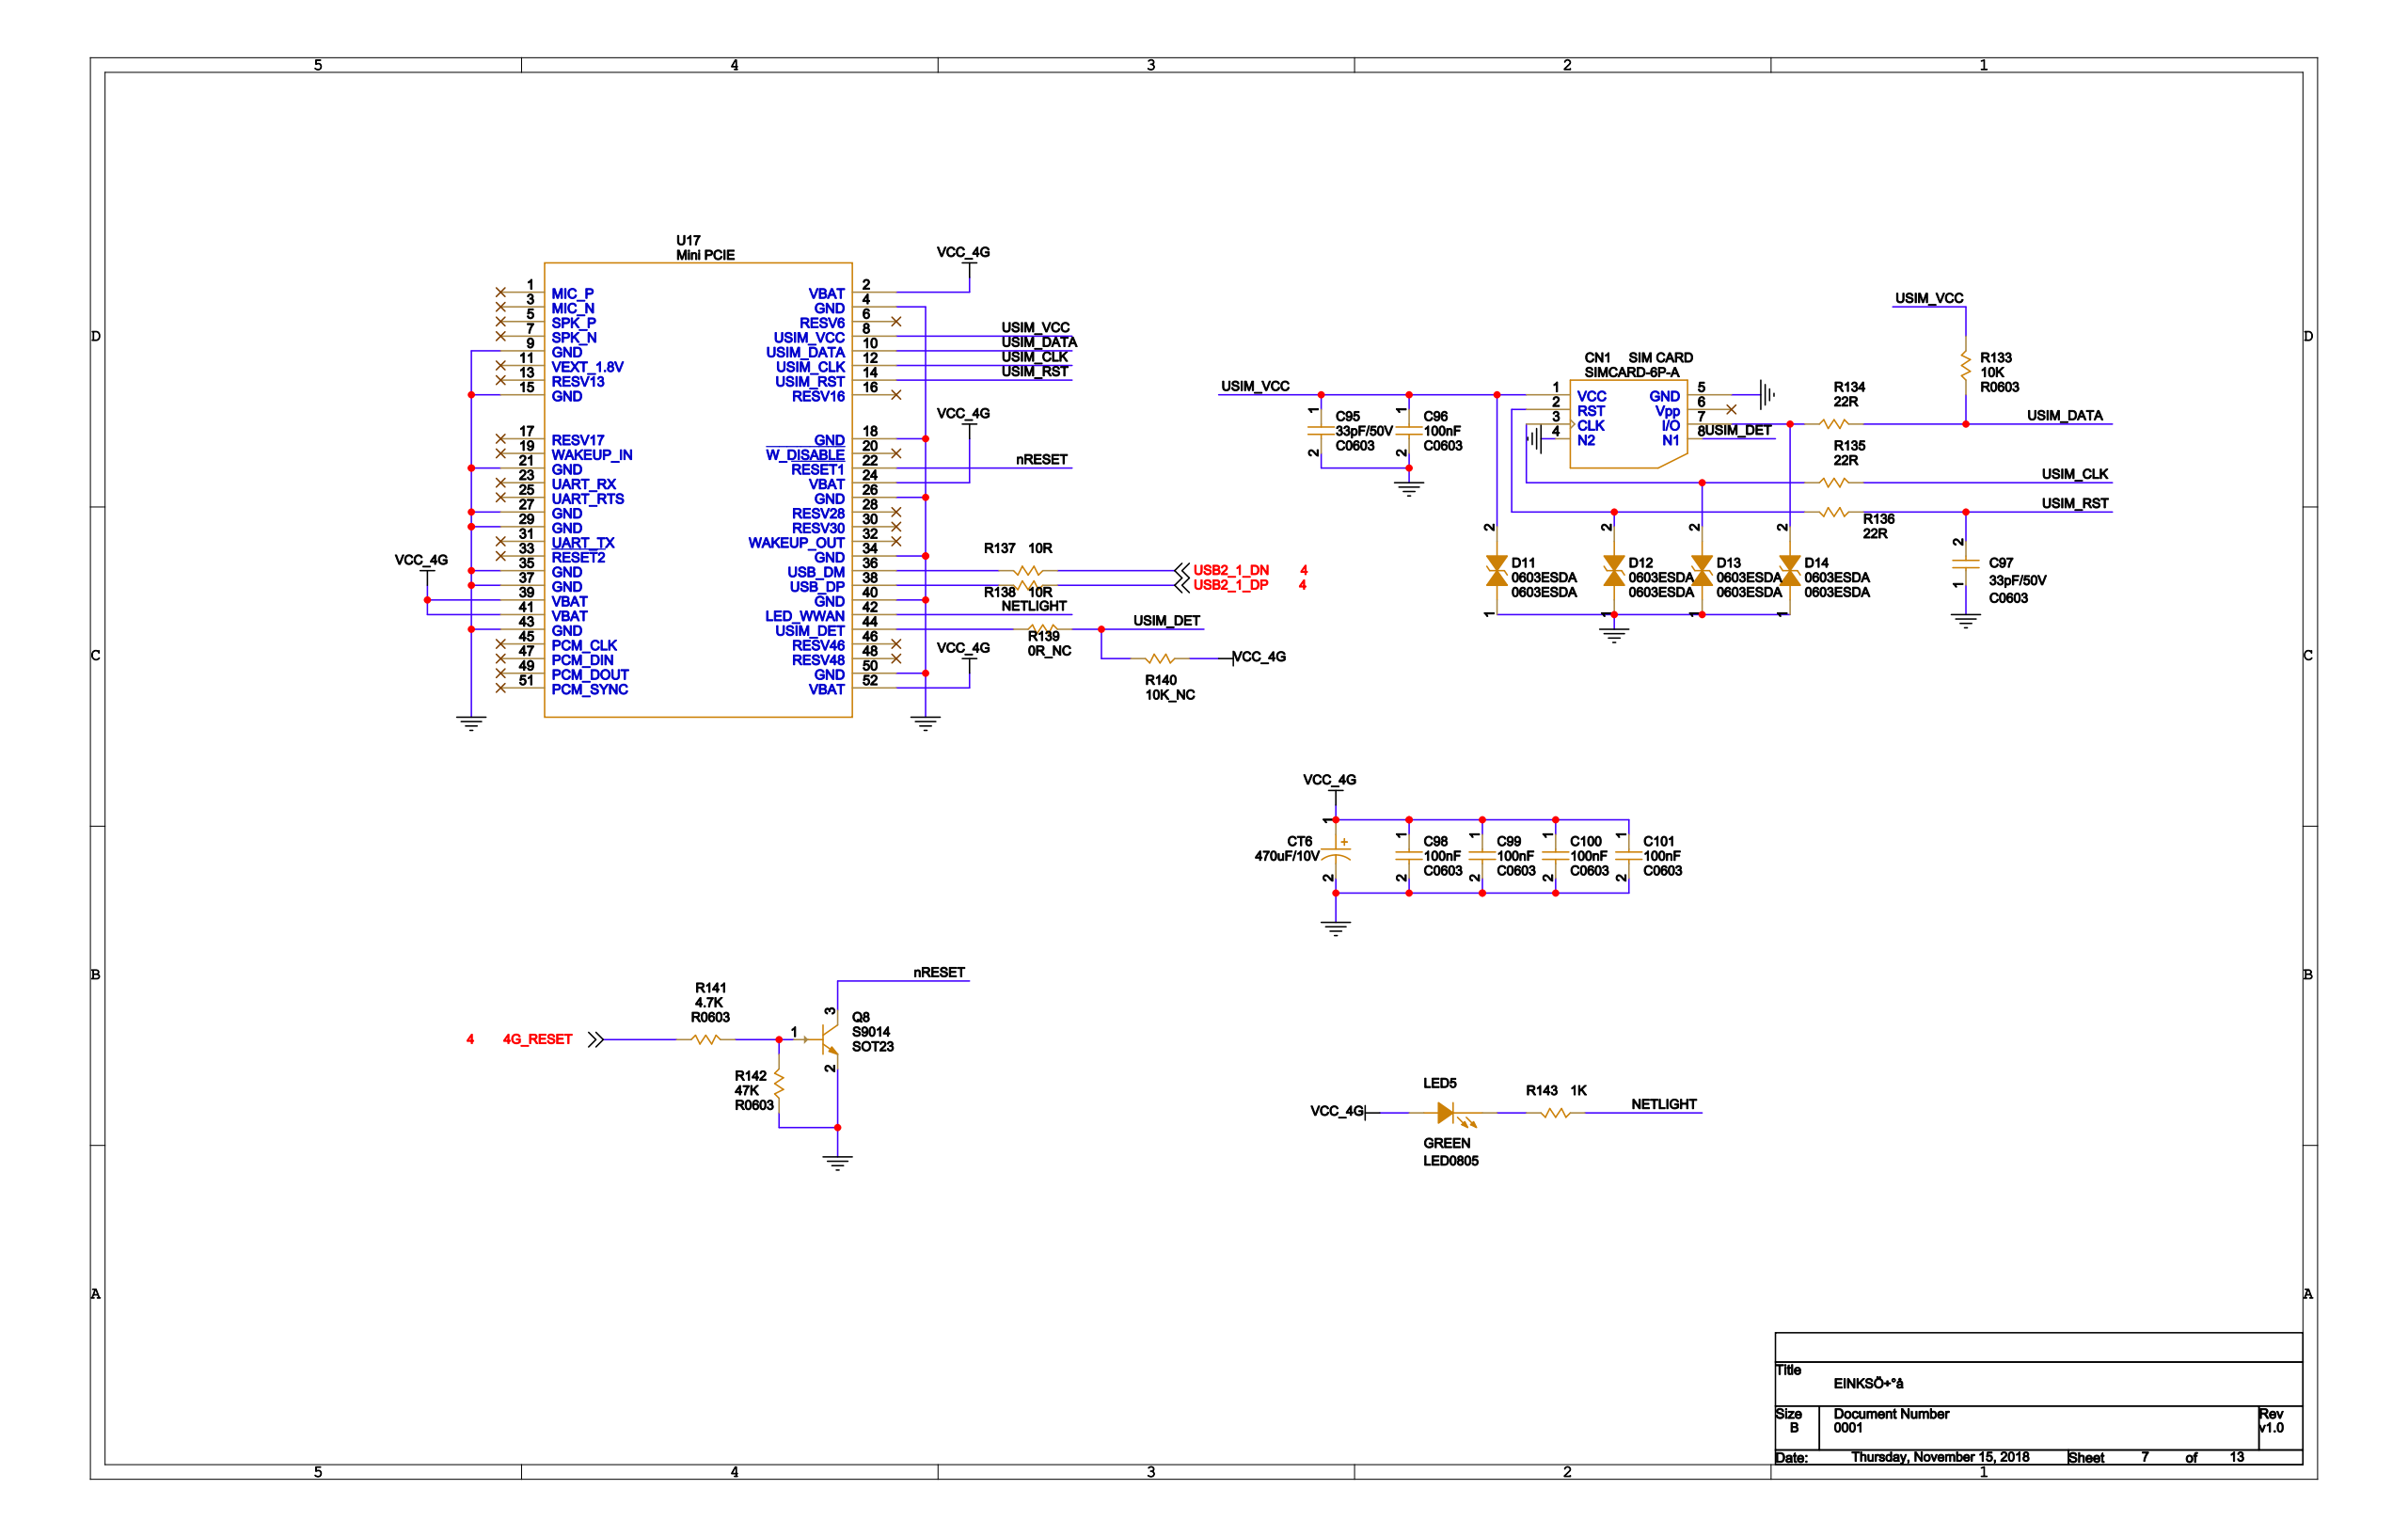Circuit board | Cadence Allegro | 609 parts | 409 nets | one sheet of the schematic
Parts on this sheet (reference | value | footprint):
C95 | 33pF/50V | C0603
C96 | 100nF | C0603
C97 | 33pF/50V | C0603
C98 | 100nF | C0603
C99 | 100nF | C0603
C100 | 100nF | C0603
C101 | 100nF | C0603
CN1 | SIM CARD | SIMCARD-6P-A
CT6 | 470uF/10V | E_CASE
D11 | 0603ESDA | 0603ESDA
D12 | 0603ESDA | 0603ESDA
D13 | 0603ESDA | 0603ESDA
D14 | 0603ESDA | 0603ESDA
LED5 | GREEN | LED0805
Q8 | S9014 | SOT23
R133 | 10K | R0603
R134 | 22R | R0603
R135 | 22R | R0603
R136 | 22R | R0603
R137 | 10R | R0603
R138 | 10R | R0603
R139 | 0R_NC | R0603
R140 | 10K_NC | R0603
R141 | 4.7K | R0603
R142 | 47K | R0603
R143 | 1K | R0603
U17 | Mini PCIE | MINI_PCIE_CON2X26_A
Nets of these parts (net: part-pin ...):
GND: C95-2 C96-2 C97-1 C98-2 C99-2 C100-2 C101-2 CN1-4 CN1-5 CT6-2 D11-1 D12-1 D13-1 D14-1 Q8-2 R142-2 U17-4 U17-9 U17-15 U17-18 U17-21 U17-26 U17-27 U17-29 U17-34 U17-35 U17-37 U17-40 U17-43 U17-50
VCC_4G: C98-1 C99-1 C100-1 C101-1 CT6-1 LED5-2 R140-1 U17-2 U17-24 U17-39 U17-41 U17-52
4G_RESET: R141-2
NETLIGHT: R143-1 U17-42
NRESET: Q8-3 U17-22
N27757630: R137-2 U17-36
N27757629: R138-2 U17-38
USIM_CLK: R135-1 U17-12
USIM_DATA: R133-1 R134-1 U17-10
N27757628: R139-2 U17-44
USIM_RST: C97-2 R136-1 U17-14
USIM_VCC: C95-1 C96-1 CN1-1 D11-2 R133-2 U17-8
USB2_1_DN: R137-1
USB2_1_DP: R138-1
N27757663: CN1-3 D13-2 R135-2
N27757671: CN1-7 D14-2 R134-2
USIM_DET: CN1-8 R139-1 R140-2
N27757669: CN1-2 D12-2 R136-2
N27757643: LED5-1 R143-2
N27757697: Q8-1 R141-1 R142-1